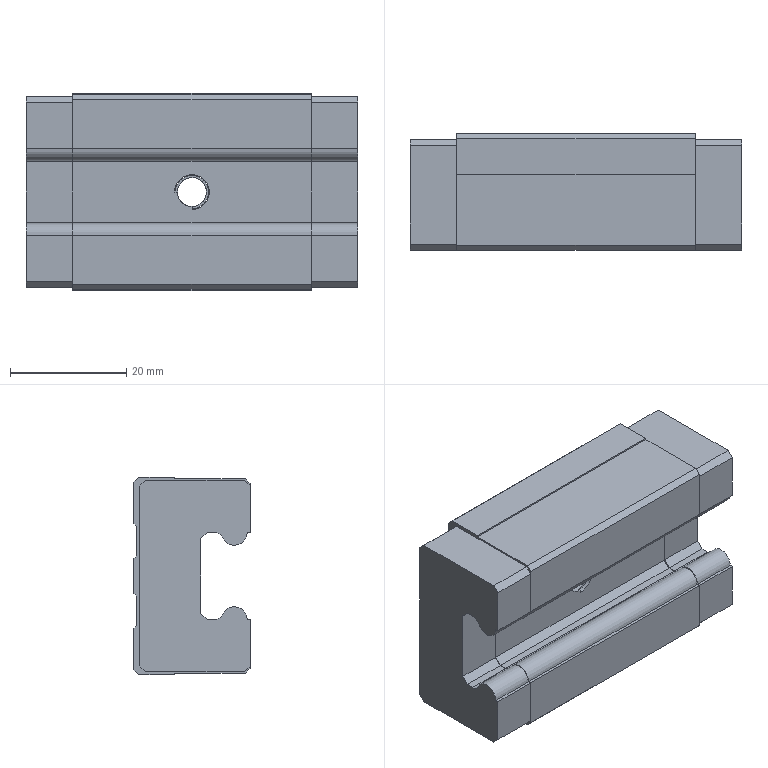Part | NX | features BREP 1 | 1 solid | 111 faces | box 57 x 20 x 34 mm | volume 30744 mm3 | plane 88 | cylinder 23 | commonest cylinder face diameters 3 x6 4.4 x6 2.9 x4 4.3 x4 5 x1 5.7 x1